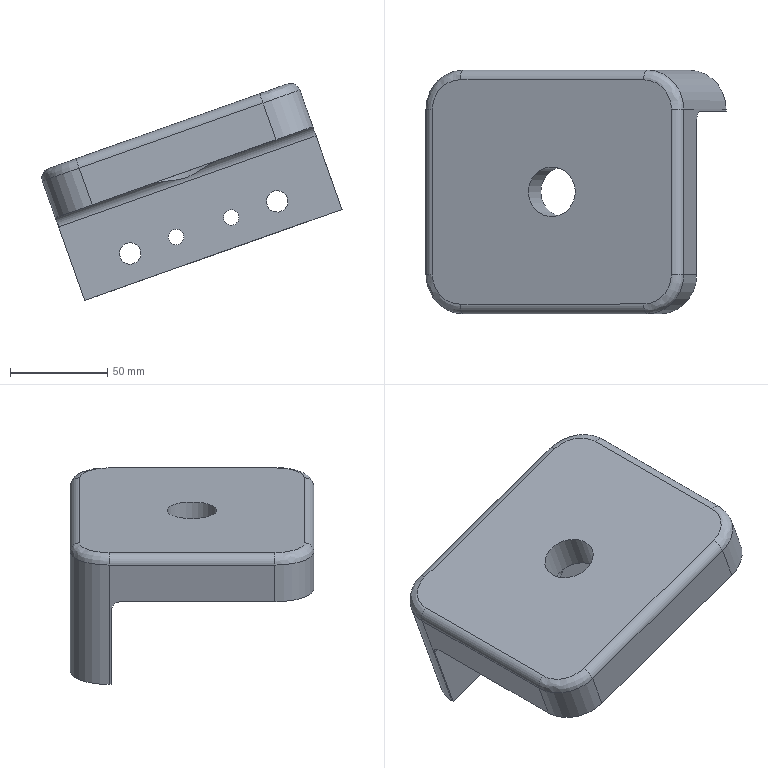Part | STEP file | MOTOR-BASE1_id426_x_t | 1 solid | 28 faces | box 155.335 x 125 x 111.336 mm | volume 504063 mm3 | cylinder 15 | plane 9 | other 4 | commonest cylinder face diameters 10 x5 40 x4 8 x2 11 x2 25.5 x1 82 x1
STEP:
#1=CARTESIAN_POINT('',(84.015,-104.8,-173.701));
#2=VERTEX_POINT('',#1);
#3=CARTESIAN_POINT('',(85.851,-104.8,-178.885));
#4=DIRECTION('',(0.,1.,0.));
#5=DIRECTION('',(-0.3338,0.,0.9426));
#6=AXIS2_PLACEMENT_3D('',#3,#4,#5);
#7=CIRCLE('',#6,5.5);
#8=EDGE_CURVE('',#2,#2,#7,.T.);
#9=ORIENTED_EDGE('',*,*,#8,.F.);
#10=EDGE_LOOP('',(#9));
#11=FACE_BOUND('',#10,.T.);
#12=CARTESIAN_POINT('',(84.015,-83.8,-173.701));
#13=VERTEX_POINT('',#12);
#14=CARTESIAN_POINT('',(85.851,-83.8,-178.885));
#15=DIRECTION('',(0.,-1.,0.));
#16=DIRECTION('',(-0.3338,0.,0.9426));
#17=AXIS2_PLACEMENT_3D('',#14,#15,#16);
#18=CIRCLE('',#17,5.5);
#19=EDGE_CURVE('',#13,#13,#18,.T.);
#20=ORIENTED_EDGE('',*,*,#19,.F.);
#21=EDGE_LOOP('',(#20));
#22=FACE_BOUND('',#21,.T.);
#23=CARTESIAN_POINT('',(85.851,-104.8,-178.885));
#24=DIRECTION('',(0.,-1.,0.));
#25=DIRECTION('',(-0.3338,0.,0.9426));
#26=AXIS2_PLACEMENT_3D('',#23,#24,#25);
#27=CYLINDRICAL_SURFACE('',#26,5.5);
#28=ADVANCED_FACE('',(#11,#22),#27,.F.);
#29=CARTESIAN_POINT('',(60.95,-104.8,-183.46));
#30=VERTEX_POINT('',#29);
#31=CARTESIAN_POINT('',(62.285,-104.8,-187.231));
#32=DIRECTION('',(0.,1.,0.));
#33=DIRECTION('',(-0.3338,0.,0.9426));
#34=AXIS2_PLACEMENT_3D('',#31,#32,#33);
#35=CIRCLE('',#34,4.);
#36=EDGE_CURVE('',#30,#30,#35,.T.);
#37=ORIENTED_EDGE('',*,*,#36,.F.);
#38=EDGE_LOOP('',(#37));
#39=FACE_BOUND('',#38,.T.);
#40=CARTESIAN_POINT('',(60.95,-83.8,-183.46));
#41=VERTEX_POINT('',#40);
#42=CARTESIAN_POINT('',(62.285,-83.8,-187.231));
#43=DIRECTION('',(0.,-1.,0.));
#44=DIRECTION('',(-0.3338,0.,0.9426));
#45=AXIS2_PLACEMENT_3D('',#42,#43,#44);
#46=CIRCLE('',#45,4.);
#47=EDGE_CURVE('',#41,#41,#46,.T.);
#48=ORIENTED_EDGE('',*,*,#47,.F.);
#49=EDGE_LOOP('',(#48));
#50=FACE_BOUND('',#49,.T.);
#51=CARTESIAN_POINT('',(62.285,-104.8,-187.231));
#52=DIRECTION('',(0.,-1.,0.));
#53=DIRECTION('',(-0.3338,0.,0.9426));
#54=AXIS2_PLACEMENT_3D('',#51,#52,#53);
#55=CYLINDRICAL_SURFACE('',#54,4.);
#56=ADVANCED_FACE('',(#39,#50),#55,.F.);
#57=CARTESIAN_POINT('',(32.67,-104.8,-193.474));
#58=VERTEX_POINT('',#57);
#59=CARTESIAN_POINT('',(34.006,-104.8,-197.245));
#60=DIRECTION('',(0.,1.,0.));
#61=DIRECTION('',(-0.3338,0.,0.9426));
#62=AXIS2_PLACEMENT_3D('',#59,#60,#61);
#63=CIRCLE('',#62,4.);
#64=EDGE_CURVE('',#58,#58,#63,.T.);
#65=ORIENTED_EDGE('',*,*,#64,.F.);
#66=EDGE_LOOP('',(#65));
#67=FACE_BOUND('',#66,.T.);
#68=CARTESIAN_POINT('',(32.67,-83.8,-193.474));
#69=VERTEX_POINT('',#68);
#70=CARTESIAN_POINT('',(34.006,-83.8,-197.245));
#71=DIRECTION('',(0.,-1.,0.));
#72=DIRECTION('',(-0.3338,0.,0.9426));
#73=AXIS2_PLACEMENT_3D('',#70,#71,#72);
#74=CIRCLE('',#73,4.);
#75=EDGE_CURVE('',#69,#69,#74,.T.);
#76=ORIENTED_EDGE('',*,*,#75,.F.);
#77=EDGE_LOOP('',(#76));
#78=FACE_BOUND('',#77,.T.);
#79=CARTESIAN_POINT('',(34.006,-104.8,-197.245));
#80=DIRECTION('',(0.,-1.,0.));
#81=DIRECTION('',(-0.3338,0.,0.9426));
#82=AXIS2_PLACEMENT_3D('',#79,#80,#81);
#83=CYLINDRICAL_SURFACE('',#82,4.);
#84=ADVANCED_FACE('',(#67,#78),#83,.F.);
#85=CARTESIAN_POINT('',(8.604,-104.8,-200.406));
#86=VERTEX_POINT('',#85);
#87=CARTESIAN_POINT('',(10.44,-104.8,-205.59));
#88=DIRECTION('',(0.,1.,0.));
#89=DIRECTION('',(-0.3338,0.,0.9426));
#90=AXIS2_PLACEMENT_3D('',#87,#88,#89);
#91=CIRCLE('',#90,5.5);
#92=EDGE_CURVE('',#86,#86,#91,.T.);
#93=ORIENTED_EDGE('',*,*,#92,.F.);
#94=EDGE_LOOP('',(#93));
#95=FACE_BOUND('',#94,.T.);
#96=CARTESIAN_POINT('',(8.604,-83.8,-200.406));
#97=VERTEX_POINT('',#96);
#98=CARTESIAN_POINT('',(10.44,-83.8,-205.59));
#99=DIRECTION('',(0.,-1.,0.));
#100=DIRECTION('',(-0.3338,0.,0.9426));
#101=AXIS2_PLACEMENT_3D('',#98,#99,#100);
#102=CIRCLE('',#101,5.5);
#103=EDGE_CURVE('',#97,#97,#102,.T.);
#104=ORIENTED_EDGE('',*,*,#103,.F.);
#105=EDGE_LOOP('',(#104));
#106=FACE_BOUND('',#105,.T.);
#107=CARTESIAN_POINT('',(10.44,-104.8,-205.59));
#108=DIRECTION('',(0.,-1.,0.));
#109=DIRECTION('',(-0.3338,0.,0.9426));
#110=AXIS2_PLACEMENT_3D('',#107,#108,#109);
#111=CYLINDRICAL_SURFACE('',#110,5.5);
#112=ADVANCED_FACE('',(#95,#106),#111,.F.);
#113=CARTESIAN_POINT('',(-12.833,-103.8,-229.744));
#114=VERTEX_POINT('',#113);
#115=CARTESIAN_POINT('',(-12.833,-104.8,-229.744));
#116=VERTEX_POINT('',#115);
#117=CARTESIAN_POINT('',(-12.833,-188.8,-229.744));
#118=DIRECTION('',(0.,-1.,0.));
#119=VECTOR('',#118,1.);
#120=LINE('',#117,#119);
#121=EDGE_CURVE('',#114,#116,#120,.T.);
#122=ORIENTED_EDGE('',*,*,#121,.F.);
#123=CARTESIAN_POINT('',(6.02,-83.8,-223.068));
#124=VERTEX_POINT('',#123);
#125=CARTESIAN_POINT('',(6.02,-103.8,-223.068));
#126=DIRECTION('',(-0.3338,0.,0.9426));
#127=DIRECTION('',(-0.9426,0.,-0.3338));
#128=AXIS2_PLACEMENT_3D('',#125,#126,#127);
#129=CIRCLE('',#128,20.);
#130=EDGE_CURVE('',#124,#114,#129,.T.);
#131=ORIENTED_EDGE('',*,*,#130,.F.);
#132=CARTESIAN_POINT('',(100.284,-83.8,-189.687));
#133=VERTEX_POINT('',#132);
#134=CARTESIAN_POINT('',(6.02,-83.8,-223.068));
#135=DIRECTION('',(-0.9426,0.,-0.3338));
#136=VECTOR('',#135,1.);
#137=LINE('',#134,#136);
#138=EDGE_CURVE('',#133,#124,#137,.T.);
#139=ORIENTED_EDGE('',*,*,#138,.F.);
#140=CARTESIAN_POINT('',(119.137,-103.8,-183.011));
#141=VERTEX_POINT('',#140);
#142=CARTESIAN_POINT('',(100.284,-103.8,-189.687));
#143=DIRECTION('',(-0.3338,0.,0.9426));
#144=DIRECTION('',(-0.9426,0.,-0.3338));
#145=AXIS2_PLACEMENT_3D('',#142,#143,#144);
#146=CIRCLE('',#145,20.);
#147=EDGE_CURVE('',#141,#133,#146,.T.);
#148=ORIENTED_EDGE('',*,*,#147,.F.);
#149=CARTESIAN_POINT('',(119.137,-104.8,-183.011));
#150=VERTEX_POINT('',#149);
#151=CARTESIAN_POINT('',(119.137,-83.8,-183.011));
#152=DIRECTION('',(0.,-1.,0.));
#153=VECTOR('',#152,1.);
#154=LINE('',#151,#153);
#155=EDGE_CURVE('',#141,#150,#154,.T.);
#156=ORIENTED_EDGE('',*,*,#155,.T.);
#157=CARTESIAN_POINT('',(119.137,-104.8,-183.011));
#158=DIRECTION('',(0.9426,0.,0.3338));
#159=VECTOR('',#158,1.);
#160=LINE('',#157,#159);
#161=EDGE_CURVE('',#116,#150,#160,.T.);
#162=ORIENTED_EDGE('',*,*,#161,.F.);
#163=EDGE_LOOP('',(#122,#131,#139,#148,#156,#162));
#164=FACE_OUTER_BOUND('',#163,.T.);
#165=CARTESIAN_POINT('',(6.02,-83.8,-223.068));
#166=DIRECTION('',(0.3338,0.,-0.9426));
#167=DIRECTION('',(-0.9426,0.,-0.3338));
#168=AXIS2_PLACEMENT_3D('',#165,#166,#167);
#169=PLANE('',#168);
#170=ADVANCED_FACE('',(#164),#169,.T.);
#171=CARTESIAN_POINT('',(20.344,-109.8,-170.257));
#172=VERTEX_POINT('',#171);
#173=CARTESIAN_POINT('',(55.918,-109.8,-157.66));
#174=VERTEX_POINT('',#173);
#175=CARTESIAN_POINT('',(38.131,-146.2,-163.959));
#176=DIRECTION('',(-0.3338,0.,0.9426));
#177=DIRECTION('',(-0.9426,0.,-0.3338));
#178=AXIS2_PLACEMENT_3D('',#175,#176,#177);
#179=CIRCLE('',#178,41.);
#180=EDGE_CURVE('',#172,#174,#179,.T.);
#181=ORIENTED_EDGE('',*,*,#180,.T.);
#182=CARTESIAN_POINT('',(104.116,-109.8,-140.592));
#183=VERTEX_POINT('',#182);
#184=CARTESIAN_POINT('',(104.406,-109.8,-140.489));
#185=DIRECTION('',(0.9426,0.,0.3338));
#186=VECTOR('',#185,1.);
#187=LINE('',#184,#186);
#188=EDGE_CURVE('',#174,#183,#187,.T.);
#189=ORIENTED_EDGE('',*,*,#188,.T.);
#190=CARTESIAN_POINT('',(104.116,-188.8,-140.592));
#191=VERTEX_POINT('',#190);
#192=CARTESIAN_POINT('',(104.116,-103.8,-140.592));
#193=DIRECTION('',(0.,1.,0.));
#194=VECTOR('',#193,1.);
#195=LINE('',#192,#194);
#196=EDGE_CURVE('',#191,#183,#195,.T.);
#197=ORIENTED_EDGE('',*,*,#196,.F.);
#198=CARTESIAN_POINT('',(85.263,-208.8,-147.268));
#199=VERTEX_POINT('',#198);
#200=CARTESIAN_POINT('',(85.263,-188.8,-147.268));
#201=DIRECTION('',(-0.3338,0.,0.9426));
#202=DIRECTION('',(-0.9426,0.,-0.3338));
#203=AXIS2_PLACEMENT_3D('',#200,#201,#202);
#204=CIRCLE('',#203,20.);
#205=EDGE_CURVE('',#199,#191,#204,.T.);
#206=ORIENTED_EDGE('',*,*,#205,.F.);
#207=CARTESIAN_POINT('',(-9.001,-208.8,-180.649));
#208=VERTEX_POINT('',#207);
#209=CARTESIAN_POINT('',(85.263,-208.8,-147.268));
#210=DIRECTION('',(0.9426,0.,0.3338));
#211=VECTOR('',#210,1.);
#212=LINE('',#209,#211);
#213=EDGE_CURVE('',#208,#199,#212,.T.);
#214=ORIENTED_EDGE('',*,*,#213,.F.);
#215=CARTESIAN_POINT('',(-27.854,-188.8,-187.325));
#216=VERTEX_POINT('',#215);
#217=CARTESIAN_POINT('',(-9.001,-188.8,-180.649));
#218=DIRECTION('',(-0.3338,0.,0.9426));
#219=DIRECTION('',(-0.9426,0.,-0.3338));
#220=AXIS2_PLACEMENT_3D('',#217,#218,#219);
#221=CIRCLE('',#220,20.);
#222=EDGE_CURVE('',#216,#208,#221,.T.);
#223=ORIENTED_EDGE('',*,*,#222,.F.);
#224=CARTESIAN_POINT('',(-27.854,-109.8,-187.325));
#225=VERTEX_POINT('',#224);
#226=CARTESIAN_POINT('',(-27.854,-188.8,-187.325));
#227=DIRECTION('',(0.,-1.,0.));
#228=VECTOR('',#227,1.);
#229=LINE('',#226,#228);
#230=EDGE_CURVE('',#225,#216,#229,.T.);
#231=ORIENTED_EDGE('',*,*,#230,.F.);
#232=CARTESIAN_POINT('',(104.406,-109.8,-140.489));
#233=DIRECTION('',(0.9426,0.,0.3338));
#234=VECTOR('',#233,1.);
#235=LINE('',#232,#234);
#236=EDGE_CURVE('',#225,#172,#235,.T.);
#237=ORIENTED_EDGE('',*,*,#236,.T.);
#238=EDGE_LOOP('',(#181,#189,#197,#206,#214,#223,#231,#237));
#239=FACE_OUTER_BOUND('',#238,.T.);
#240=CARTESIAN_POINT('',(38.131,-146.2,-163.959));
#241=DIRECTION('',(0.3338,0.,-0.9426));
#242=DIRECTION('',(-0.9426,0.,-0.3338));
#243=AXIS2_PLACEMENT_3D('',#240,#241,#242);
#244=PLANE('',#243);
#245=ADVANCED_FACE('',(#239),#244,.T.);
#246=ORIENTED_EDGE('',*,*,#188,.F.);
#247=CARTESIAN_POINT('',(55.918,-109.8,-157.66));
#248=CARTESIAN_POINT('',(53.104,-108.253,-158.656));
#249=CARTESIAN_POINT('',(50.42,-107.116,-160.297));
#250=CARTESIAN_POINT('',(46.312,-105.967,-162.914));
#251=CARTESIAN_POINT('',(44.944,-105.681,-163.817));
#252=CARTESIAN_POINT('',(42.11,-105.295,-165.517));
#253=CARTESIAN_POINT('',(40.611,-105.196,-166.316));
#254=CARTESIAN_POINT('',(35.931,-105.208,-167.942));
#255=CARTESIAN_POINT('',(32.58,-105.611,-168.126));
#256=CARTESIAN_POINT('',(26.218,-107.138,-168.856));
#257=CARTESIAN_POINT('',(23.159,-108.252,-169.26));
#258=CARTESIAN_POINT('',(20.344,-109.8,-170.257));
#259=B_SPLINE_CURVE_WITH_KNOTS('',3,(#247,#248,#249,#250,#251,#252,#253,#254,#255,#256,#257,#258),.UNSPECIFIED.,.F.,.F.,(4,2,2,2,2,4),(0.,0.25,0.375,0.5,0.75,1.),.UNSPECIFIED.);
#260=EDGE_CURVE('',#174,#172,#259,.T.);
#261=ORIENTED_EDGE('',*,*,#260,.T.);
#262=ORIENTED_EDGE('',*,*,#236,.F.);
#263=CARTESIAN_POINT('',(-26.185,-104.8,-192.038));
#264=VERTEX_POINT('',#263);
#265=CARTESIAN_POINT('',(-26.185,-109.8,-192.038));
#266=DIRECTION('',(0.9426,0.,0.3338));
#267=DIRECTION('',(-0.3338,0.,0.9426));
#268=AXIS2_PLACEMENT_3D('',#265,#266,#267);
#269=CIRCLE('',#268,5.);
#270=EDGE_CURVE('',#264,#225,#269,.T.);
#271=ORIENTED_EDGE('',*,*,#270,.F.);
#272=CARTESIAN_POINT('',(105.785,-104.8,-145.305));
#273=VERTEX_POINT('',#272);
#274=CARTESIAN_POINT('',(105.785,-104.8,-145.305));
#275=DIRECTION('',(-0.9426,0.,-0.3338));
#276=VECTOR('',#275,1.);
#277=LINE('',#274,#276);
#278=EDGE_CURVE('',#273,#264,#277,.T.);
#279=ORIENTED_EDGE('',*,*,#278,.F.);
#280=CARTESIAN_POINT('',(105.785,-109.8,-145.305));
#281=DIRECTION('',(-0.9426,0.,-0.3338));
#282=DIRECTION('',(-0.3338,0.,0.9426));
#283=AXIS2_PLACEMENT_3D('',#280,#281,#282);
#284=CIRCLE('',#283,5.);
#285=EDGE_CURVE('',#183,#273,#284,.T.);
#286=ORIENTED_EDGE('',*,*,#285,.F.);
#287=EDGE_LOOP('',(#246,#261,#262,#271,#279,#286));
#288=FACE_OUTER_BOUND('',#287,.T.);
#289=CARTESIAN_POINT('',(106.075,-109.8,-145.202));
#290=DIRECTION('',(-0.9426,0.,-0.3338));
#291=DIRECTION('',(-0.3338,0.,0.9426));
#292=AXIS2_PLACEMENT_3D('',#289,#290,#291);
#293=CYLINDRICAL_SURFACE('',#292,5.);
#294=ADVANCED_FACE('',(#288),#293,.F.);
#295=ORIENTED_EDGE('',*,*,#92,.T.);
#296=EDGE_LOOP('',(#295));
#297=FACE_BOUND('',#296,.T.);
#298=ORIENTED_EDGE('',*,*,#64,.T.);
#299=EDGE_LOOP('',(#298));
#300=FACE_BOUND('',#299,.T.);
#301=ORIENTED_EDGE('',*,*,#36,.T.);
#302=EDGE_LOOP('',(#301));
#303=FACE_BOUND('',#302,.T.);
#304=ORIENTED_EDGE('',*,*,#8,.T.);
#305=EDGE_LOOP('',(#304));
#306=FACE_BOUND('',#305,.T.);
#307=CARTESIAN_POINT('',(95.771,-104.8,-117.026));
#308=DIRECTION('',(0.3338,0.,-0.9426));
#309=VECTOR('',#308,1.);
#310=LINE('',#307,#309);
#311=EDGE_CURVE('',#273,#150,#310,.T.);
#312=ORIENTED_EDGE('',*,*,#311,.F.);
#313=ORIENTED_EDGE('',*,*,#278,.T.);
#314=CARTESIAN_POINT('',(-36.199,-104.8,-163.759));
#315=DIRECTION('',(-0.3338,0.,0.9426));
#316=VECTOR('',#315,1.);
#317=LINE('',#314,#316);
#318=EDGE_CURVE('',#116,#264,#317,.T.);
#319=ORIENTED_EDGE('',*,*,#318,.F.);
#320=ORIENTED_EDGE('',*,*,#161,.T.);
#321=EDGE_LOOP('',(#312,#313,#319,#320));
#322=FACE_BOUND('',#321,.T.);
#323=CARTESIAN_POINT('',(104.116,-104.8,-140.592));
#324=DIRECTION('',(0.,-1.,0.));
#325=DIRECTION('',(-0.3338,0.,0.9426));
#326=AXIS2_PLACEMENT_3D('',#323,#324,#325);
#327=PLANE('',#326);
#328=ADVANCED_FACE('',(#297,#300,#303,#306,#322),#327,.T.);
#329=CARTESIAN_POINT('',(-2.52,-146.2,-171.989));
#330=VERTEX_POINT('',#329);
#331=CARTESIAN_POINT('',(36.128,-146.2,-158.303));
#332=DIRECTION('',(0.3338,0.,-0.9426));
#333=DIRECTION('',(-0.9426,0.,-0.3338));
#334=AXIS2_PLACEMENT_3D('',#331,#332,#333);
#335=CIRCLE('',#334,41.);
#336=EDGE_CURVE('',#330,#330,#335,.T.);
#337=ORIENTED_EDGE('',*,*,#336,.F.);
#338=EDGE_LOOP('',(#337));
#339=FACE_BOUND('',#338,.T.);
#340=ORIENTED_EDGE('',*,*,#260,.F.);
#341=ORIENTED_EDGE('',*,*,#180,.F.);
#342=EDGE_LOOP('',(#340,#341));
#343=FACE_BOUND('',#342,.T.);
#344=CARTESIAN_POINT('',(38.131,-146.2,-163.959));
#345=DIRECTION('',(0.3338,0.,-0.9426));
#346=DIRECTION('',(-0.9426,0.,-0.3338));
#347=AXIS2_PLACEMENT_3D('',#344,#345,#346);
#348=CYLINDRICAL_SURFACE('',#347,41.);
#349=ADVANCED_FACE('',(#339,#343),#348,.F.);
#350=CARTESIAN_POINT('',(97.44,-188.8,-121.739));
#351=VERTEX_POINT('',#350);
#352=CARTESIAN_POINT('',(95.771,-188.8,-117.026));
#353=DIRECTION('',(0.3338,0.,-0.9426));
#354=VECTOR('',#353,1.);
#355=LINE('',#352,#354);
#356=EDGE_CURVE('',#351,#191,#355,.T.);
#357=ORIENTED_EDGE('',*,*,#356,.F.);
#358=CARTESIAN_POINT('',(78.587,-208.8,-128.415));
#359=VERTEX_POINT('',#358);
#360=CARTESIAN_POINT('',(78.587,-188.8,-128.415));
#361=DIRECTION('',(-0.3338,0.,0.9426));
#362=DIRECTION('',(-0.01949,-0.9998,-0.006902));
#363=AXIS2_PLACEMENT_3D('',#360,#361,#362);
#364=CIRCLE('',#363,20.);
#365=EDGE_CURVE('',#359,#351,#364,.T.);
#366=ORIENTED_EDGE('',*,*,#365,.F.);
#367=CARTESIAN_POINT('',(76.918,-208.8,-123.702));
#368=DIRECTION('',(-0.3338,0.,0.9426));
#369=VECTOR('',#368,1.);
#370=LINE('',#367,#369);
#371=EDGE_CURVE('',#199,#359,#370,.T.);
#372=ORIENTED_EDGE('',*,*,#371,.F.);
#373=ORIENTED_EDGE('',*,*,#205,.T.);
#374=EDGE_LOOP('',(#357,#366,#372,#373));
#375=FACE_OUTER_BOUND('',#374,.T.);
#376=CARTESIAN_POINT('',(76.918,-188.8,-123.702));
#377=DIRECTION('',(0.3338,0.,-0.9426));
#378=DIRECTION('',(-0.9426,0.,-0.3338));
#379=AXIS2_PLACEMENT_3D('',#376,#377,#378);
#380=CYLINDRICAL_SURFACE('',#379,20.);
#381=ADVANCED_FACE('',(#375),#380,.T.);
#382=ORIENTED_EDGE('',*,*,#371,.T.);
#383=CARTESIAN_POINT('',(-15.677,-208.8,-161.796));
#384=VERTEX_POINT('',#383);
#385=CARTESIAN_POINT('',(-16.067,-208.8,-161.934));
#386=DIRECTION('',(0.9426,0.,0.3338));
#387=VECTOR('',#386,1.);
#388=LINE('',#385,#387);
#389=EDGE_CURVE('',#384,#359,#388,.T.);
#390=ORIENTED_EDGE('',*,*,#389,.F.);
#391=CARTESIAN_POINT('',(-17.346,-208.8,-157.083));
#392=DIRECTION('',(-0.3338,0.,0.9426));
#393=VECTOR('',#392,1.);
#394=LINE('',#391,#393);
#395=EDGE_CURVE('',#208,#384,#394,.T.);
#396=ORIENTED_EDGE('',*,*,#395,.F.);
#397=ORIENTED_EDGE('',*,*,#213,.T.);
#398=EDGE_LOOP('',(#382,#390,#396,#397));
#399=FACE_OUTER_BOUND('',#398,.T.);
#400=CARTESIAN_POINT('',(76.918,-208.8,-123.702));
#401=DIRECTION('',(0.,-1.,0.));
#402=DIRECTION('',(-0.3338,0.,0.9426));
#403=AXIS2_PLACEMENT_3D('',#400,#401,#402);
#404=PLANE('',#403);
#405=ADVANCED_FACE('',(#399),#404,.T.);
#406=ORIENTED_EDGE('',*,*,#395,.T.);
#407=CARTESIAN_POINT('',(-34.53,-188.8,-168.472));
#408=VERTEX_POINT('',#407);
#409=CARTESIAN_POINT('',(-15.677,-188.8,-161.796));
#410=DIRECTION('',(-0.3338,0.,0.9426));
#411=DIRECTION('',(-0.9424,0.02068,-0.3337));
#412=AXIS2_PLACEMENT_3D('',#409,#410,#411);
#413=CIRCLE('',#412,20.);
#414=EDGE_CURVE('',#408,#384,#413,.T.);
#415=ORIENTED_EDGE('',*,*,#414,.F.);
#416=CARTESIAN_POINT('',(-36.199,-188.8,-163.759));
#417=DIRECTION('',(-0.3338,0.,0.9426));
#418=VECTOR('',#417,1.);
#419=LINE('',#416,#418);
#420=EDGE_CURVE('',#216,#408,#419,.T.);
#421=ORIENTED_EDGE('',*,*,#420,.F.);
#422=ORIENTED_EDGE('',*,*,#222,.T.);
#423=EDGE_LOOP('',(#406,#415,#421,#422));
#424=FACE_OUTER_BOUND('',#423,.T.);
#425=CARTESIAN_POINT('',(-17.346,-188.8,-157.083));
#426=DIRECTION('',(0.3338,0.,-0.9426));
#427=DIRECTION('',(-0.9426,0.,-0.3338));
#428=AXIS2_PLACEMENT_3D('',#425,#426,#427);
#429=CYLINDRICAL_SURFACE('',#428,20.);
#430=ADVANCED_FACE('',(#424),#429,.T.);
#431=ORIENTED_EDGE('',*,*,#270,.T.);
#432=ORIENTED_EDGE('',*,*,#230,.T.);
#433=ORIENTED_EDGE('',*,*,#420,.T.);
#434=CARTESIAN_POINT('',(-34.53,-103.8,-168.472));
#435=VERTEX_POINT('',#434);
#436=CARTESIAN_POINT('',(-34.53,-103.386,-168.472));
#437=DIRECTION('',(0.,-1.,0.));
#438=VECTOR('',#437,1.);
#439=LINE('',#436,#438);
#440=EDGE_CURVE('',#435,#408,#439,.T.);
#441=ORIENTED_EDGE('',*,*,#440,.F.);
#442=CARTESIAN_POINT('',(-36.199,-103.8,-163.759));
#443=DIRECTION('',(-0.3338,0.,0.9426));
#444=VECTOR('',#443,1.);
#445=LINE('',#442,#444);
#446=EDGE_CURVE('',#114,#435,#445,.T.);
#447=ORIENTED_EDGE('',*,*,#446,.F.);
#448=ORIENTED_EDGE('',*,*,#121,.T.);
#449=ORIENTED_EDGE('',*,*,#318,.T.);
#450=EDGE_LOOP('',(#431,#432,#433,#441,#447,#448,#449));
#451=FACE_OUTER_BOUND('',#450,.T.);
#452=CARTESIAN_POINT('',(-36.199,-188.8,-163.759));
#453=DIRECTION('',(-0.9426,0.,-0.3338));
#454=DIRECTION('',(-0.3338,0.,0.9426));
#455=AXIS2_PLACEMENT_3D('',#452,#453,#454);
#456=PLANE('',#455);
#457=ADVANCED_FACE('',(#451),#456,.T.);
#458=ORIENTED_EDGE('',*,*,#130,.T.);
#459=ORIENTED_EDGE('',*,*,#446,.T.);
#460=CARTESIAN_POINT('',(-15.677,-83.8,-161.796));
#461=VERTEX_POINT('',#460);
#462=CARTESIAN_POINT('',(-15.677,-103.8,-161.796));
#463=DIRECTION('',(-0.3338,0.,0.9426));
#464=DIRECTION('',(0.01949,0.9998,0.006902));
#465=AXIS2_PLACEMENT_3D('',#462,#463,#464);
#466=CIRCLE('',#465,20.);
#467=EDGE_CURVE('',#461,#435,#466,.T.);
#468=ORIENTED_EDGE('',*,*,#467,.F.);
#469=CARTESIAN_POINT('',(-17.346,-83.8,-157.083));
#470=DIRECTION('',(-0.3338,0.,0.9426));
#471=VECTOR('',#470,1.);
#472=LINE('',#469,#471);
#473=EDGE_CURVE('',#124,#461,#472,.T.);
#474=ORIENTED_EDGE('',*,*,#473,.F.);
#475=EDGE_LOOP('',(#458,#459,#468,#474));
#476=FACE_OUTER_BOUND('',#475,.T.);
#477=CARTESIAN_POINT('',(-17.346,-103.8,-157.083));
#478=DIRECTION('',(0.3338,0.,-0.9426));
#479=DIRECTION('',(-0.9426,0.,-0.3338));
#480=AXIS2_PLACEMENT_3D('',#477,#478,#479);
#481=CYLINDRICAL_SURFACE('',#480,20.);
#482=ADVANCED_FACE('',(#476),#481,.T.);
#483=ORIENTED_EDGE('',*,*,#103,.T.);
#484=EDGE_LOOP('',(#483));
#485=FACE_BOUND('',#484,.T.);
#486=ORIENTED_EDGE('',*,*,#75,.T.);
#487=EDGE_LOOP('',(#486));
#488=FACE_BOUND('',#487,.T.);
#489=ORIENTED_EDGE('',*,*,#47,.T.);
#490=EDGE_LOOP('',(#489));
#491=FACE_BOUND('',#490,.T.);
#492=ORIENTED_EDGE('',*,*,#19,.T.);
#493=EDGE_LOOP('',(#492));
#494=FACE_BOUND('',#493,.T.);
#495=ORIENTED_EDGE('',*,*,#138,.T.);
#496=ORIENTED_EDGE('',*,*,#473,.T.);
#497=CARTESIAN_POINT('',(78.587,-83.8,-128.415));
#498=VERTEX_POINT('',#497);
#499=CARTESIAN_POINT('',(78.977,-83.8,-128.277));
#500=DIRECTION('',(-0.9426,0.,-0.3338));
#501=VECTOR('',#500,1.);
#502=LINE('',#499,#501);
#503=EDGE_CURVE('',#498,#461,#502,.T.);
#504=ORIENTED_EDGE('',*,*,#503,.F.);
#505=CARTESIAN_POINT('',(76.918,-83.8,-123.702));
#506=DIRECTION('',(-0.3338,0.,0.9426));
#507=VECTOR('',#506,1.);
#508=LINE('',#505,#507);
#509=EDGE_CURVE('',#133,#498,#508,.T.);
#510=ORIENTED_EDGE('',*,*,#509,.F.);
#511=EDGE_LOOP('',(#495,#496,#504,#510));
#512=FACE_BOUND('',#511,.T.);
#513=CARTESIAN_POINT('',(-17.346,-83.8,-157.083));
#514=DIRECTION('',(0.,1.,0.));
#515=DIRECTION('',(0.3338,0.,-0.9426));
#516=AXIS2_PLACEMENT_3D('',#513,#514,#515);
#517=PLANE('',#516);
#518=ADVANCED_FACE('',(#485,#488,#491,#494,#512),#517,.T.);
#519=ORIENTED_EDGE('',*,*,#147,.T.);
#520=ORIENTED_EDGE('',*,*,#509,.T.);
#521=CARTESIAN_POINT('',(97.44,-103.8,-121.739));
#522=VERTEX_POINT('',#521);
#523=CARTESIAN_POINT('',(78.587,-103.8,-128.415));
#524=DIRECTION('',(-0.3338,0.,0.9426));
#525=DIRECTION('',(0.9424,-0.02068,0.3337));
#526=AXIS2_PLACEMENT_3D('',#523,#524,#525);
#527=CIRCLE('',#526,20.);
#528=EDGE_CURVE('',#522,#498,#527,.T.);
#529=ORIENTED_EDGE('',*,*,#528,.F.);
#530=CARTESIAN_POINT('',(95.771,-103.8,-117.026));
#531=DIRECTION('',(-0.3338,0.,0.9426));
#532=VECTOR('',#531,1.);
#533=LINE('',#530,#532);
#534=EDGE_CURVE('',#141,#522,#533,.T.);
#535=ORIENTED_EDGE('',*,*,#534,.F.);
#536=EDGE_LOOP('',(#519,#520,#529,#535));
#537=FACE_OUTER_BOUND('',#536,.T.);
#538=CARTESIAN_POINT('',(76.918,-103.8,-123.702));
#539=DIRECTION('',(0.3338,0.,-0.9426));
#540=DIRECTION('',(-0.9426,0.,-0.3338));
#541=AXIS2_PLACEMENT_3D('',#538,#539,#540);
#542=CYLINDRICAL_SURFACE('',#541,20.);
#543=ADVANCED_FACE('',(#537),#542,.T.);
#544=ORIENTED_EDGE('',*,*,#285,.T.);
#545=ORIENTED_EDGE('',*,*,#311,.T.);
#546=ORIENTED_EDGE('',*,*,#155,.F.);
#547=ORIENTED_EDGE('',*,*,#534,.T.);
#548=CARTESIAN_POINT('',(97.44,-189.214,-121.739));
#549=DIRECTION('',(0.,1.,0.));
#550=VECTOR('',#549,1.);
#551=LINE('',#548,#550);
#552=EDGE_CURVE('',#351,#522,#551,.T.);
#553=ORIENTED_EDGE('',*,*,#552,.F.);
#554=ORIENTED_EDGE('',*,*,#356,.T.);
#555=ORIENTED_EDGE('',*,*,#196,.T.);
#556=EDGE_LOOP('',(#544,#545,#546,#547,#553,#554,#555));
#557=FACE_OUTER_BOUND('',#556,.T.);
#558=CARTESIAN_POINT('',(95.771,-103.8,-117.026));
#559=DIRECTION('',(0.9426,0.,0.3338));
#560=DIRECTION('',(0.3338,0.,-0.9426));
#561=AXIS2_PLACEMENT_3D('',#558,#559,#560);
#562=PLANE('',#561);
#563=ADVANCED_FACE('',(#557),#562,.T.);
#564=CARTESIAN_POINT('',(24.109,-146.2,-162.559));
#565=VERTEX_POINT('',#564);
#566=CARTESIAN_POINT('',(36.128,-146.2,-158.303));
#567=DIRECTION('',(-0.3338,0.,0.9426));
#568=DIRECTION('',(-0.9426,0.,-0.3338));
#569=AXIS2_PLACEMENT_3D('',#566,#567,#568);
#570=CIRCLE('',#569,12.75);
#571=EDGE_CURVE('',#565,#565,#570,.T.);
#572=ORIENTED_EDGE('',*,*,#571,.T.);
#573=EDGE_LOOP('',(#572));
#574=FACE_BOUND('',#573,.T.);
#575=ORIENTED_EDGE('',*,*,#336,.T.);
#576=EDGE_LOOP('',(#575));
#577=FACE_BOUND('',#576,.T.);
#578=CARTESIAN_POINT('',(-11.004,-83.8,-174.993));
#579=DIRECTION('',(0.3338,0.,-0.9426));
#580=DIRECTION('',(-0.9426,0.,-0.3338));
#581=AXIS2_PLACEMENT_3D('',#578,#579,#580);
#582=PLANE('',#581);
#583=ADVANCED_FACE('',(#574,#577),#582,.T.);
#584=CARTESIAN_POINT('',(91.057,-188.8,-118.695));
#585=VERTEX_POINT('',#584);
#586=CARTESIAN_POINT('',(92.727,-188.8,-123.408));
#587=DIRECTION('',(0.,1.,0.));
#588=DIRECTION('',(0.3338,0.,-0.9426));
#589=AXIS2_PLACEMENT_3D('',#586,#587,#588);
#590=CIRCLE('',#589,5.);
#591=EDGE_CURVE('',#585,#351,#590,.T.);
#592=ORIENTED_EDGE('',*,*,#591,.F.);
#593=CARTESIAN_POINT('',(76.918,-203.8,-123.702));
#594=VERTEX_POINT('',#593);
#595=CARTESIAN_POINT('',(91.057,-188.8,-118.695));
#596=CARTESIAN_POINT('',(91.057,-197.587,-118.695));
#597=CARTESIAN_POINT('',(85.201,-203.8,-120.769));
#598=CARTESIAN_POINT('',(76.918,-203.8,-123.702));
#599=(BOUNDED_CURVE()B_SPLINE_CURVE(3,(#595,#596,#597,#598),.UNSPECIFIED.,.F.,.F.)B_SPLINE_CURVE_WITH_KNOTS((4,4),(0.,1.),.UNSPECIFIED.)CURVE()GEOMETRIC_REPRESENTATION_ITEM()RATIONAL_B_SPLINE_CURVE((1.,0.8047,0.8047,1.))REPRESENTATION_ITEM(''));
#600=EDGE_CURVE('',#585,#594,#599,.T.);
#601=ORIENTED_EDGE('',*,*,#600,.T.);
#602=CARTESIAN_POINT('',(78.587,-203.8,-128.415));
#603=DIRECTION('',(-0.9426,0.,-0.3338));
#604=DIRECTION('',(0.3338,0.,-0.9426));
#605=AXIS2_PLACEMENT_3D('',#602,#603,#604);
#606=CIRCLE('',#605,5.);
#607=EDGE_CURVE('',#359,#594,#606,.T.);
#608=ORIENTED_EDGE('',*,*,#607,.F.);
#609=ORIENTED_EDGE('',*,*,#365,.T.);
#610=EDGE_LOOP('',(#592,#601,#608,#609));
#611=FACE_OUTER_BOUND('',#610,.T.);
#612=CARTESIAN_POINT('',(78.295,-203.797,-128.519));
#613=DIRECTION('',(-0.9424,0.02068,-0.3337));
#614=DIRECTION('',(-0.01949,-0.9998,-0.006902));
#615=AXIS2_PLACEMENT_3D('',#612,#613,#614);
#616=CIRCLE('',#615,5.);
#617=CARTESIAN_POINT('',(78.587,-188.8,-128.415));
#618=DIRECTION('',(0.3338,0.,-0.9426));
#619=AXIS1_PLACEMENT('',#617,#618);
#620=SURFACE_OF_REVOLUTION('',#616,#619);
#621=ADVANCED_FACE('',(#611),#620,.F.);
#622=ORIENTED_EDGE('',*,*,#607,.T.);
#623=CARTESIAN_POINT('',(-17.346,-203.8,-157.083));
#624=VERTEX_POINT('',#623);
#625=CARTESIAN_POINT('',(29.786,-203.8,-140.392));
#626=DIRECTION('',(-0.9426,0.,-0.3338));
#627=VECTOR('',#626,1.);
#628=LINE('',#625,#627);
#629=EDGE_CURVE('',#594,#624,#628,.T.);
#630=ORIENTED_EDGE('',*,*,#629,.T.);
#631=CARTESIAN_POINT('',(-15.677,-203.8,-161.796));
#632=DIRECTION('',(-0.9426,0.,-0.3338));
#633=DIRECTION('',(0.,-1.,0.));
#634=AXIS2_PLACEMENT_3D('',#631,#632,#633);
#635=CIRCLE('',#634,5.);
#636=EDGE_CURVE('',#384,#624,#635,.T.);
#637=ORIENTED_EDGE('',*,*,#636,.F.);
#638=ORIENTED_EDGE('',*,*,#389,.T.);
#639=EDGE_LOOP('',(#622,#630,#637,#638));
#640=FACE_OUTER_BOUND('',#639,.T.);
#641=CARTESIAN_POINT('',(-16.067,-203.8,-161.934));
#642=DIRECTION('',(0.9426,0.,0.3338));
#643=DIRECTION('',(0.3338,0.,-0.9426));
#644=AXIS2_PLACEMENT_3D('',#641,#642,#643);
#645=CYLINDRICAL_SURFACE('',#644,5.);
#646=ADVANCED_FACE('',(#640),#645,.T.);
#647=ORIENTED_EDGE('',*,*,#636,.T.);
#648=CARTESIAN_POINT('',(-31.486,-188.8,-162.09));
#649=VERTEX_POINT('',#648);
#650=CARTESIAN_POINT('',(-17.346,-203.8,-157.083));
#651=CARTESIAN_POINT('',(-25.629,-203.8,-160.016));
#652=CARTESIAN_POINT('',(-31.486,-197.587,-162.09));
#653=CARTESIAN_POINT('',(-31.486,-188.8,-162.09));
#654=(BOUNDED_CURVE()B_SPLINE_CURVE(3,(#650,#651,#652,#653),.UNSPECIFIED.,.F.,.F.)B_SPLINE_CURVE_WITH_KNOTS((4,4),(0.,1.),.UNSPECIFIED.)CURVE()GEOMETRIC_REPRESENTATION_ITEM()RATIONAL_B_SPLINE_CURVE((1.,0.8047,0.8047,1.))REPRESENTATION_ITEM(''));
#655=EDGE_CURVE('',#624,#649,#654,.T.);
#656=ORIENTED_EDGE('',*,*,#655,.T.);
#657=CARTESIAN_POINT('',(-29.817,-188.8,-166.803));
#658=DIRECTION('',(0.,1.,0.));
#659=DIRECTION('',(-0.3338,0.,0.9426));
#660=AXIS2_PLACEMENT_3D('',#657,#658,#659);
#661=CIRCLE('',#660,5.);
#662=EDGE_CURVE('',#408,#649,#661,.T.);
#663=ORIENTED_EDGE('',*,*,#662,.F.);
#664=ORIENTED_EDGE('',*,*,#414,.T.);
#665=EDGE_LOOP('',(#647,#656,#663,#664));
#666=FACE_OUTER_BOUND('',#665,.T.);
#667=CARTESIAN_POINT('',(-29.814,-188.49,-166.802));
#668=DIRECTION('',(0.01949,0.9998,0.006902));
#669=DIRECTION('',(-0.9424,0.02068,-0.3337));
#670=AXIS2_PLACEMENT_3D('',#667,#668,#669);
#671=CIRCLE('',#670,5.);
#672=CARTESIAN_POINT('',(-15.677,-188.8,-161.796));
#673=DIRECTION('',(0.3338,0.,-0.9426));
#674=AXIS1_PLACEMENT('',#672,#673);
#675=SURFACE_OF_REVOLUTION('',#671,#674);
#676=ADVANCED_FACE('',(#666),#675,.F.);
#677=ORIENTED_EDGE('',*,*,#662,.T.);
#678=CARTESIAN_POINT('',(-31.486,-103.8,-162.09));
#679=VERTEX_POINT('',#678);
#680=CARTESIAN_POINT('',(-31.486,-146.2,-162.09));
#681=DIRECTION('',(0.,1.,0.));
#682=VECTOR('',#681,1.);
#683=LINE('',#680,#682);
#684=EDGE_CURVE('',#649,#679,#683,.T.);
#685=ORIENTED_EDGE('',*,*,#684,.T.);
#686=CARTESIAN_POINT('',(-29.817,-103.8,-166.803));
#687=DIRECTION('',(0.,1.,0.));
#688=DIRECTION('',(-0.9426,0.,-0.3338));
#689=AXIS2_PLACEMENT_3D('',#686,#687,#688);
#690=CIRCLE('',#689,5.);
#691=EDGE_CURVE('',#435,#679,#690,.T.);
#692=ORIENTED_EDGE('',*,*,#691,.F.);
#693=ORIENTED_EDGE('',*,*,#440,.T.);
#694=EDGE_LOOP('',(#677,#685,#692,#693));
#695=FACE_OUTER_BOUND('',#694,.T.);
#696=CARTESIAN_POINT('',(-29.817,-103.386,-166.803));
#697=DIRECTION('',(0.,-1.,0.));
#698=DIRECTION('',(-0.3338,0.,0.9426));
#699=AXIS2_PLACEMENT_3D('',#696,#697,#698);
#700=CYLINDRICAL_SURFACE('',#699,5.);
#701=ADVANCED_FACE('',(#695),#700,.T.);
#702=ORIENTED_EDGE('',*,*,#691,.T.);
#703=CARTESIAN_POINT('',(-17.346,-88.8,-157.083));
#704=VERTEX_POINT('',#703);
#705=CARTESIAN_POINT('',(-31.486,-103.8,-162.09));
#706=CARTESIAN_POINT('',(-31.486,-95.013,-162.09));
#707=CARTESIAN_POINT('',(-25.629,-88.8,-160.016));
#708=CARTESIAN_POINT('',(-17.346,-88.8,-157.083));
#709=(BOUNDED_CURVE()B_SPLINE_CURVE(3,(#705,#706,#707,#708),.UNSPECIFIED.,.F.,.F.)B_SPLINE_CURVE_WITH_KNOTS((4,4),(0.,1.),.UNSPECIFIED.)CURVE()GEOMETRIC_REPRESENTATION_ITEM()RATIONAL_B_SPLINE_CURVE((1.,0.8047,0.8047,1.))REPRESENTATION_ITEM(''));
#710=EDGE_CURVE('',#679,#704,#709,.T.);
#711=ORIENTED_EDGE('',*,*,#710,.T.);
#712=CARTESIAN_POINT('',(-15.677,-88.8,-161.796));
#713=DIRECTION('',(0.9426,0.,0.3338));
#714=DIRECTION('',(-0.3338,0.,0.9426));
#715=AXIS2_PLACEMENT_3D('',#712,#713,#714);
#716=CIRCLE('',#715,5.);
#717=EDGE_CURVE('',#461,#704,#716,.T.);
#718=ORIENTED_EDGE('',*,*,#717,.F.);
#719=ORIENTED_EDGE('',*,*,#467,.T.);
#720=EDGE_LOOP('',(#702,#711,#718,#719));
#721=FACE_OUTER_BOUND('',#720,.T.);
#722=CARTESIAN_POINT('',(-15.385,-88.803,-161.693));
#723=DIRECTION('',(0.9424,-0.02068,0.3337));
#724=DIRECTION('',(0.01949,0.9998,0.006902));
#725=AXIS2_PLACEMENT_3D('',#722,#723,#724);
#726=CIRCLE('',#725,5.);
#727=CARTESIAN_POINT('',(-15.677,-103.8,-161.796));
#728=DIRECTION('',(0.3338,0.,-0.9426));
#729=AXIS1_PLACEMENT('',#727,#728);
#730=SURFACE_OF_REVOLUTION('',#726,#729);
#731=ADVANCED_FACE('',(#721),#730,.F.);
#732=ORIENTED_EDGE('',*,*,#717,.T.);
#733=CARTESIAN_POINT('',(76.918,-88.8,-123.702));
#734=VERTEX_POINT('',#733);
#735=CARTESIAN_POINT('',(29.786,-88.8,-140.392));
#736=DIRECTION('',(0.9426,0.,0.3338));
#737=VECTOR('',#736,1.);
#738=LINE('',#735,#737);
#739=EDGE_CURVE('',#704,#734,#738,.T.);
#740=ORIENTED_EDGE('',*,*,#739,.T.);
#741=CARTESIAN_POINT('',(78.587,-88.8,-128.415));
#742=DIRECTION('',(0.9426,0.,0.3338));
#743=DIRECTION('',(0.,1.,0.));
#744=AXIS2_PLACEMENT_3D('',#741,#742,#743);
#745=CIRCLE('',#744,5.);
#746=EDGE_CURVE('',#498,#734,#745,.T.);
#747=ORIENTED_EDGE('',*,*,#746,.F.);
#748=ORIENTED_EDGE('',*,*,#503,.T.);
#749=EDGE_LOOP('',(#732,#740,#747,#748));
#750=FACE_OUTER_BOUND('',#749,.T.);
#751=CARTESIAN_POINT('',(78.977,-88.8,-128.277));
#752=DIRECTION('',(-0.9426,0.,-0.3338));
#753=DIRECTION('',(-0.3338,0.,0.9426));
#754=AXIS2_PLACEMENT_3D('',#751,#752,#753);
#755=CYLINDRICAL_SURFACE('',#754,5.);
#756=ADVANCED_FACE('',(#750),#755,.T.);
#757=ORIENTED_EDGE('',*,*,#746,.T.);
#758=CARTESIAN_POINT('',(91.057,-103.8,-118.695));
#759=VERTEX_POINT('',#758);
#760=CARTESIAN_POINT('',(76.918,-88.8,-123.702));
#761=CARTESIAN_POINT('',(85.201,-88.8,-120.769));
#762=CARTESIAN_POINT('',(91.057,-95.013,-118.695));
#763=CARTESIAN_POINT('',(91.057,-103.8,-118.695));
#764=(BOUNDED_CURVE()B_SPLINE_CURVE(3,(#760,#761,#762,#763),.UNSPECIFIED.,.F.,.F.)B_SPLINE_CURVE_WITH_KNOTS((4,4),(0.,1.),.UNSPECIFIED.)CURVE()GEOMETRIC_REPRESENTATION_ITEM()RATIONAL_B_SPLINE_CURVE((1.,0.8047,0.8047,1.))REPRESENTATION_ITEM(''));
#765=EDGE_CURVE('',#734,#759,#764,.T.);
#766=ORIENTED_EDGE('',*,*,#765,.T.);
#767=CARTESIAN_POINT('',(92.727,-103.8,-123.408));
#768=DIRECTION('',(0.,-1.,0.));
#769=DIRECTION('',(0.3338,0.,-0.9426));
#770=AXIS2_PLACEMENT_3D('',#767,#768,#769);
#771=CIRCLE('',#770,5.);
#772=EDGE_CURVE('',#522,#759,#771,.T.);
#773=ORIENTED_EDGE('',*,*,#772,.F.);
#774=ORIENTED_EDGE('',*,*,#528,.T.);
#775=EDGE_LOOP('',(#757,#766,#773,#774));
#776=FACE_OUTER_BOUND('',#775,.T.);
#777=CARTESIAN_POINT('',(92.723,-104.11,-123.409));
#778=DIRECTION('',(-0.01949,-0.9998,-0.006902));
#779=DIRECTION('',(0.9424,-0.02068,0.3337));
#780=AXIS2_PLACEMENT_3D('',#777,#778,#779);
#781=CIRCLE('',#780,5.);
#782=CARTESIAN_POINT('',(78.587,-103.8,-128.415));
#783=DIRECTION('',(0.3338,0.,-0.9426));
#784=AXIS1_PLACEMENT('',#782,#783);
#785=SURFACE_OF_REVOLUTION('',#781,#784);
#786=ADVANCED_FACE('',(#776),#785,.F.);
#787=ORIENTED_EDGE('',*,*,#772,.T.);
#788=CARTESIAN_POINT('',(91.057,-146.2,-118.695));
#789=DIRECTION('',(0.,-1.,0.));
#790=VECTOR('',#789,1.);
#791=LINE('',#788,#790);
#792=EDGE_CURVE('',#759,#585,#791,.T.);
#793=ORIENTED_EDGE('',*,*,#792,.T.);
#794=ORIENTED_EDGE('',*,*,#591,.T.);
#795=ORIENTED_EDGE('',*,*,#552,.T.);
#796=EDGE_LOOP('',(#787,#793,#794,#795));
#797=FACE_OUTER_BOUND('',#796,.T.);
#798=CARTESIAN_POINT('',(92.727,-189.214,-123.408));
#799=DIRECTION('',(0.,1.,0.));
#800=DIRECTION('',(0.3338,0.,-0.9426));
#801=AXIS2_PLACEMENT_3D('',#798,#799,#800);
#802=CYLINDRICAL_SURFACE('',#801,5.);
#803=ADVANCED_FACE('',(#797),#802,.T.);
#804=ORIENTED_EDGE('',*,*,#571,.F.);
#805=EDGE_LOOP('',(#804));
#806=FACE_BOUND('',#805,.T.);
#807=CARTESIAN_POINT('',(17.767,-146.2,-144.649));
#808=VERTEX_POINT('',#807);
#809=CARTESIAN_POINT('',(29.786,-146.2,-140.392));
#810=DIRECTION('',(-0.3338,0.,0.9426));
#811=DIRECTION('',(-0.9426,0.,-0.3338));
#812=AXIS2_PLACEMENT_3D('',#809,#810,#811);
#813=CIRCLE('',#812,12.75);
#814=EDGE_CURVE('',#808,#808,#813,.T.);
#815=ORIENTED_EDGE('',*,*,#814,.T.);
#816=EDGE_LOOP('',(#815));
#817=FACE_BOUND('',#816,.T.);
#818=CARTESIAN_POINT('',(38.131,-146.2,-163.959));
#819=DIRECTION('',(0.3338,0.,-0.9426));
#820=DIRECTION('',(-0.9426,0.,-0.3338));
#821=AXIS2_PLACEMENT_3D('',#818,#819,#820);
#822=CYLINDRICAL_SURFACE('',#821,12.75);
#823=ADVANCED_FACE('',(#806,#817),#822,.F.);
#824=ORIENTED_EDGE('',*,*,#814,.F.);
#825=EDGE_LOOP('',(#824));
#826=FACE_BOUND('',#825,.T.);
#827=ORIENTED_EDGE('',*,*,#765,.F.);
#828=ORIENTED_EDGE('',*,*,#739,.F.);
#829=ORIENTED_EDGE('',*,*,#710,.F.);
#830=ORIENTED_EDGE('',*,*,#684,.F.);
#831=ORIENTED_EDGE('',*,*,#655,.F.);
#832=ORIENTED_EDGE('',*,*,#629,.F.);
#833=ORIENTED_EDGE('',*,*,#600,.F.);
#834=ORIENTED_EDGE('',*,*,#792,.F.);
#835=EDGE_LOOP('',(#827,#828,#829,#830,#831,#832,#833,#834));
#836=FACE_BOUND('',#835,.T.);
#837=CARTESIAN_POINT('',(29.786,-146.2,-140.392));
#838=DIRECTION('',(0.3338,0.,-0.9426));
#839=DIRECTION('',(-0.9426,0.,-0.3338));
#840=AXIS2_PLACEMENT_3D('',#837,#838,#839);
#841=PLANE('',#840);
#842=ADVANCED_FACE('',(#826,#836),#841,.F.);
#843=CLOSED_SHELL('',(#28,#56,#84,#112,#170,#245,#294,#328,#349,#381,#405,#430,#457,#482,#518,#543,#563,#583,#621,#646,#676,#701,#731,#756,#786,#803,#823,#842));
#844=MANIFOLD_SOLID_BREP('',#843);
#845=(LENGTH_UNIT()NAMED_UNIT(*)SI_UNIT(.MILLI.,.METRE.));
#846=UNCERTAINTY_MEASURE_WITH_UNIT(LENGTH_MEASURE(0.0508),#845,'','');
#847=(NAMED_UNIT(*)PLANE_ANGLE_UNIT()SI_UNIT($,.RADIAN.));
#848=PLANE_ANGLE_MEASURE_WITH_UNIT(PLANE_ANGLE_MEASURE(0.01745),#847);
#849=DIMENSIONAL_EXPONENTS(0.,0.,0.,0.,0.,0.,0.);
#850=(CONVERSION_BASED_UNIT('DEGREE',#848)NAMED_UNIT(#849)PLANE_ANGLE_UNIT());
#851=(NAMED_UNIT(*)SI_UNIT($,.STERADIAN.)SOLID_ANGLE_UNIT());
#852=(GEOMETRIC_REPRESENTATION_CONTEXT(3)GLOBAL_UNCERTAINTY_ASSIGNED_CONTEXT((#846))GLOBAL_UNIT_ASSIGNED_CONTEXT((#845,#850,#851))REPRESENTATION_CONTEXT('',''));
#853=ADVANCED_BREP_SHAPE_REPRESENTATION('',(#844),#852);